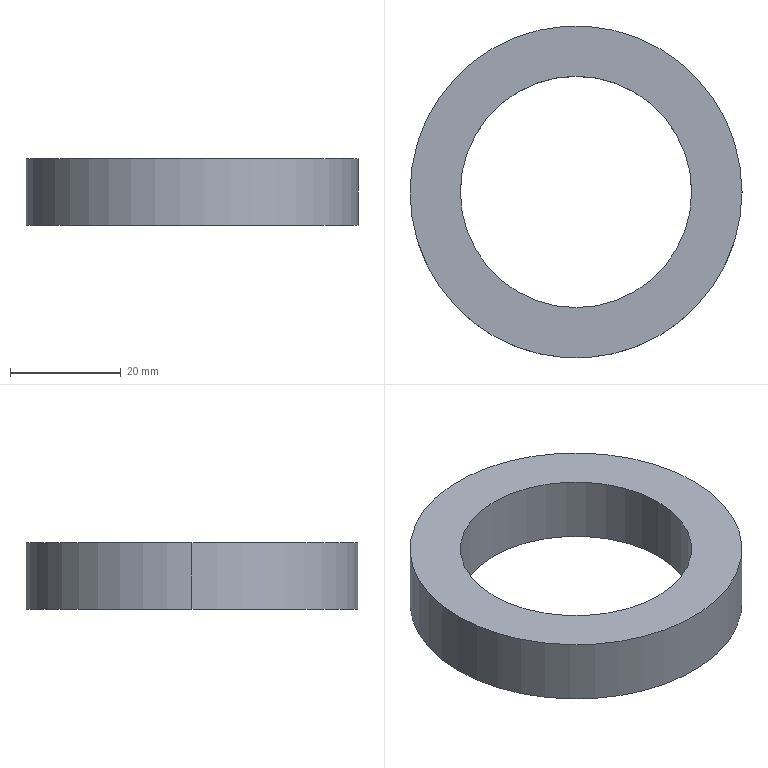Part | SolidWorks | features Extrusion 1 | 1 solid | 6 faces | box 60 x 60 x 12 mm | volume 17462 mm3 | cylinder 4 | plane 2 | commonest cylinder face diameters 41.8 x2 60 x2
STEP:
#1=CARTESIAN_POINT('',(-20.9,0.,12.));
#2=VERTEX_POINT('',#1);
#3=CARTESIAN_POINT('',(20.9,0.,12.));
#4=VERTEX_POINT('',#3);
#5=CARTESIAN_POINT('',(0.,0.,12.));
#6=DIRECTION('',(0.,0.,1.));
#7=DIRECTION('',(1.,0.,0.));
#8=AXIS2_PLACEMENT_3D('',#5,#6,#7);
#9=CIRCLE('',#8,20.9);
#10=EDGE_CURVE('',#2,#4,#9,.T.);
#11=ORIENTED_EDGE('',*,*,#10,.T.);
#12=CARTESIAN_POINT('',(20.9,0.,0.));
#13=VERTEX_POINT('',#12);
#14=CARTESIAN_POINT('',(20.9,0.,12.));
#15=DIRECTION('',(0.,0.,-1.));
#16=VECTOR('',#15,1000.);
#17=LINE('',#14,#16);
#18=EDGE_CURVE('',#4,#13,#17,.T.);
#19=ORIENTED_EDGE('',*,*,#18,.T.);
#20=CARTESIAN_POINT('',(-20.9,0.,0.));
#21=VERTEX_POINT('',#20);
#22=CARTESIAN_POINT('',(0.,0.,0.));
#23=DIRECTION('',(0.,0.,1.));
#24=DIRECTION('',(1.,0.,0.));
#25=AXIS2_PLACEMENT_3D('',#22,#23,#24);
#26=CIRCLE('',#25,20.9);
#27=EDGE_CURVE('',#21,#13,#26,.T.);
#28=ORIENTED_EDGE('',*,*,#27,.F.);
#29=CARTESIAN_POINT('',(-20.9,0.,12.));
#30=DIRECTION('',(0.,0.,-1.));
#31=VECTOR('',#30,1000.);
#32=LINE('',#29,#31);
#33=EDGE_CURVE('',#2,#21,#32,.T.);
#34=ORIENTED_EDGE('',*,*,#33,.F.);
#35=EDGE_LOOP('',(#11,#19,#28,#34));
#36=FACE_OUTER_BOUND('',#35,.T.);
#37=CARTESIAN_POINT('',(0.,0.,12.));
#38=DIRECTION('',(0.,0.,-1.));
#39=DIRECTION('',(-1.,0.,0.));
#40=AXIS2_PLACEMENT_3D('',#37,#38,#39);
#41=CYLINDRICAL_SURFACE('',#40,20.9);
#42=ADVANCED_FACE('',(#36),#41,.F.);
#43=CARTESIAN_POINT('',(30.,0.,12.));
#44=VERTEX_POINT('',#43);
#45=CARTESIAN_POINT('',(-30.,0.,12.));
#46=VERTEX_POINT('',#45);
#47=CARTESIAN_POINT('',(0.,0.,12.));
#48=DIRECTION('',(0.,0.,1.));
#49=DIRECTION('',(1.,0.,0.));
#50=AXIS2_PLACEMENT_3D('',#47,#48,#49);
#51=CIRCLE('',#50,30.);
#52=EDGE_CURVE('',#44,#46,#51,.T.);
#53=ORIENTED_EDGE('',*,*,#52,.F.);
#54=CARTESIAN_POINT('',(30.,0.,0.));
#55=VERTEX_POINT('',#54);
#56=CARTESIAN_POINT('',(30.,0.,12.));
#57=DIRECTION('',(0.,0.,-1.));
#58=VECTOR('',#57,1000.);
#59=LINE('',#56,#58);
#60=EDGE_CURVE('',#44,#55,#59,.T.);
#61=ORIENTED_EDGE('',*,*,#60,.T.);
#62=CARTESIAN_POINT('',(-30.,0.,0.));
#63=VERTEX_POINT('',#62);
#64=CARTESIAN_POINT('',(0.,0.,0.));
#65=DIRECTION('',(0.,0.,1.));
#66=DIRECTION('',(1.,0.,0.));
#67=AXIS2_PLACEMENT_3D('',#64,#65,#66);
#68=CIRCLE('',#67,30.);
#69=EDGE_CURVE('',#55,#63,#68,.T.);
#70=ORIENTED_EDGE('',*,*,#69,.T.);
#71=CARTESIAN_POINT('',(-30.,0.,12.));
#72=DIRECTION('',(0.,0.,-1.));
#73=VECTOR('',#72,1000.);
#74=LINE('',#71,#73);
#75=EDGE_CURVE('',#46,#63,#74,.T.);
#76=ORIENTED_EDGE('',*,*,#75,.F.);
#77=EDGE_LOOP('',(#53,#61,#70,#76));
#78=FACE_OUTER_BOUND('',#77,.T.);
#79=CARTESIAN_POINT('',(0.,0.,12.));
#80=DIRECTION('',(0.,0.,-1.));
#81=DIRECTION('',(-1.,0.,0.));
#82=AXIS2_PLACEMENT_3D('',#79,#80,#81);
#83=CYLINDRICAL_SURFACE('',#82,30.);
#84=ADVANCED_FACE('',(#78),#83,.T.);
#85=CARTESIAN_POINT('',(0.,0.,12.));
#86=DIRECTION('',(0.,0.,1.));
#87=DIRECTION('',(1.,0.,0.));
#88=AXIS2_PLACEMENT_3D('',#85,#86,#87);
#89=CIRCLE('',#88,30.);
#90=EDGE_CURVE('',#46,#44,#89,.T.);
#91=ORIENTED_EDGE('',*,*,#90,.T.);
#92=ORIENTED_EDGE('',*,*,#52,.T.);
#93=EDGE_LOOP('',(#91,#92));
#94=FACE_OUTER_BOUND('',#93,.T.);
#95=ORIENTED_EDGE('',*,*,#10,.F.);
#96=CARTESIAN_POINT('',(0.,0.,12.));
#97=DIRECTION('',(0.,0.,1.));
#98=DIRECTION('',(1.,0.,0.));
#99=AXIS2_PLACEMENT_3D('',#96,#97,#98);
#100=CIRCLE('',#99,20.9);
#101=EDGE_CURVE('',#4,#2,#100,.T.);
#102=ORIENTED_EDGE('',*,*,#101,.F.);
#103=EDGE_LOOP('',(#95,#102));
#104=FACE_BOUND('',#103,.T.);
#105=CARTESIAN_POINT('',(0.,0.,12.));
#106=DIRECTION('',(0.,0.,1.));
#107=DIRECTION('',(1.,0.,0.));
#108=AXIS2_PLACEMENT_3D('',#105,#106,#107);
#109=PLANE('',#108);
#110=ADVANCED_FACE('',(#94,#104),#109,.T.);
#111=CARTESIAN_POINT('',(0.,0.,0.));
#112=DIRECTION('',(0.,0.,1.));
#113=DIRECTION('',(1.,0.,0.));
#114=AXIS2_PLACEMENT_3D('',#111,#112,#113);
#115=CIRCLE('',#114,30.);
#116=EDGE_CURVE('',#63,#55,#115,.T.);
#117=ORIENTED_EDGE('',*,*,#116,.F.);
#118=ORIENTED_EDGE('',*,*,#69,.F.);
#119=EDGE_LOOP('',(#117,#118));
#120=FACE_OUTER_BOUND('',#119,.T.);
#121=ORIENTED_EDGE('',*,*,#27,.T.);
#122=CARTESIAN_POINT('',(0.,0.,0.));
#123=DIRECTION('',(0.,0.,1.));
#124=DIRECTION('',(1.,0.,0.));
#125=AXIS2_PLACEMENT_3D('',#122,#123,#124);
#126=CIRCLE('',#125,20.9);
#127=EDGE_CURVE('',#13,#21,#126,.T.);
#128=ORIENTED_EDGE('',*,*,#127,.T.);
#129=EDGE_LOOP('',(#121,#128));
#130=FACE_BOUND('',#129,.T.);
#131=CARTESIAN_POINT('',(0.,0.,0.));
#132=DIRECTION('',(0.,0.,1.));
#133=DIRECTION('',(1.,0.,0.));
#134=AXIS2_PLACEMENT_3D('',#131,#132,#133);
#135=PLANE('',#134);
#136=ADVANCED_FACE('',(#120,#130),#135,.F.);
#137=ORIENTED_EDGE('',*,*,#60,.F.);
#138=ORIENTED_EDGE('',*,*,#90,.F.);
#139=ORIENTED_EDGE('',*,*,#75,.T.);
#140=ORIENTED_EDGE('',*,*,#116,.T.);
#141=EDGE_LOOP('',(#137,#138,#139,#140));
#142=FACE_OUTER_BOUND('',#141,.T.);
#143=CARTESIAN_POINT('',(0.,0.,12.));
#144=DIRECTION('',(0.,0.,-1.));
#145=DIRECTION('',(-1.,0.,0.));
#146=AXIS2_PLACEMENT_3D('',#143,#144,#145);
#147=CYLINDRICAL_SURFACE('',#146,30.);
#148=ADVANCED_FACE('',(#142),#147,.T.);
#149=ORIENTED_EDGE('',*,*,#18,.F.);
#150=ORIENTED_EDGE('',*,*,#101,.T.);
#151=ORIENTED_EDGE('',*,*,#33,.T.);
#152=ORIENTED_EDGE('',*,*,#127,.F.);
#153=EDGE_LOOP('',(#149,#150,#151,#152));
#154=FACE_OUTER_BOUND('',#153,.T.);
#155=CARTESIAN_POINT('',(0.,0.,12.));
#156=DIRECTION('',(0.,0.,-1.));
#157=DIRECTION('',(-1.,0.,0.));
#158=AXIS2_PLACEMENT_3D('',#155,#156,#157);
#159=CYLINDRICAL_SURFACE('',#158,20.9);
#160=ADVANCED_FACE('',(#154),#159,.F.);
#161=CLOSED_SHELL('',(#42,#84,#110,#136,#148,#160));
#162=MANIFOLD_SOLID_BREP('',#161);
#163=CARTESIAN_POINT('',(0.,0.,0.));
#164=DIRECTION('',(0.,0.,1.));
#165=DIRECTION('',(1.,0.,0.));
#166=AXIS2_PLACEMENT_3D('',#163,#164,#165);
#167=(LENGTH_UNIT()NAMED_UNIT(*)SI_UNIT(.MILLI.,.METRE.));
#168=UNCERTAINTY_MEASURE_WITH_UNIT(LENGTH_MEASURE(0.00001),#167,'','');
#169=(NAMED_UNIT(*)PLANE_ANGLE_UNIT()SI_UNIT($,.RADIAN.));
#170=(NAMED_UNIT(*)SI_UNIT($,.STERADIAN.)SOLID_ANGLE_UNIT());
#171=(GEOMETRIC_REPRESENTATION_CONTEXT(3)GLOBAL_UNCERTAINTY_ASSIGNED_CONTEXT((#168))GLOBAL_UNIT_ASSIGNED_CONTEXT((#167,#169,#170))REPRESENTATION_CONTEXT('',''));
#172=ADVANCED_BREP_SHAPE_REPRESENTATION('',(#162,#166),#171);